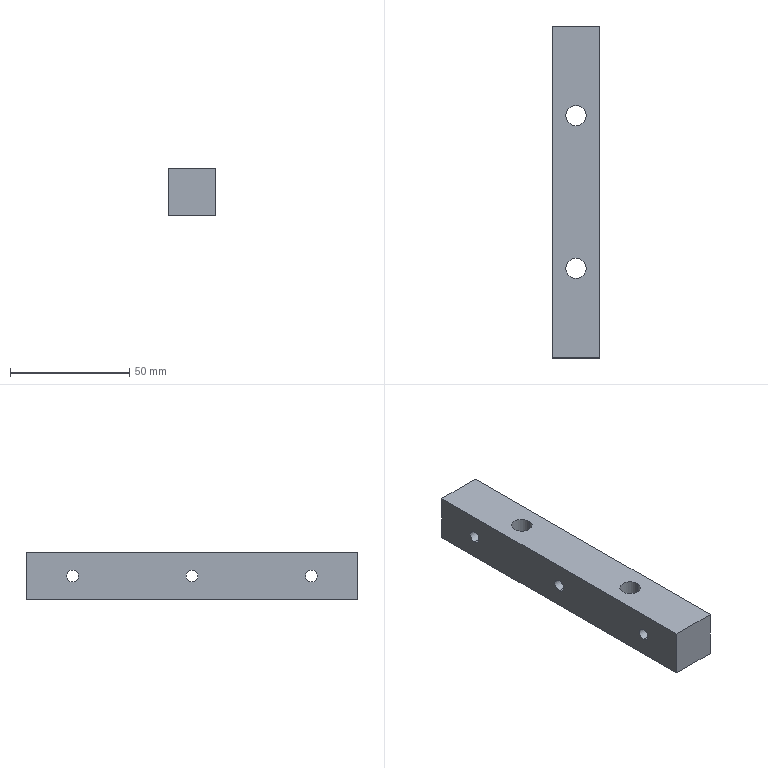Part | STEP file | 1 solid | 26 faces | box 20 x 139 x 20 mm | volume 52128 mm3 | cone 10 | cylinder 10 | plane 6 | commonest cylinder face diameters 5 x6 8.5 x4